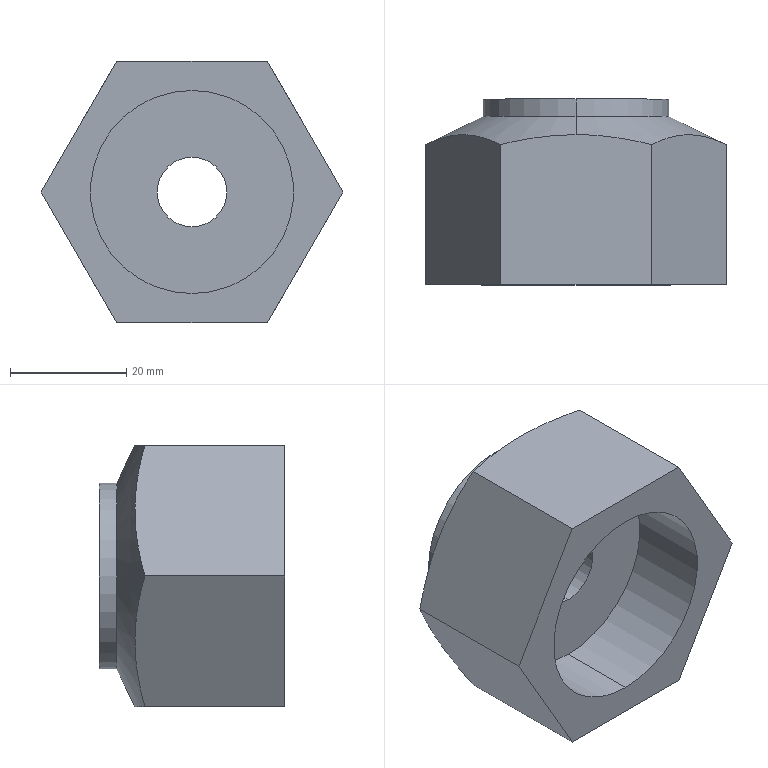Part | SolidWorks | features ICE 7 | 1 solid | 20 faces | box 51.962 x 32 x 45 mm | volume 33727 mm3 | plane 10 | cylinder 8 | cone 2 | commonest cylinder face diameters 12 x2 18 x2 32 x2 35 x2
STEP:
#1=CARTESIAN_POINT('',(0.,5.,-16.));
#2=VERTEX_POINT('',#1);
#3=CARTESIAN_POINT('',(0.,5.,16.));
#4=VERTEX_POINT('',#3);
#5=CARTESIAN_POINT('',(0.,5.,0.));
#6=DIRECTION('',(0.,1.,0.));
#7=DIRECTION('',(0.,0.,1.));
#8=AXIS2_PLACEMENT_3D('',#5,#6,#7);
#9=CIRCLE('',#8,16.);
#10=EDGE_CURVE('',#2,#4,#9,.T.);
#11=ORIENTED_EDGE('',*,*,#10,.F.);
#12=CARTESIAN_POINT('',(0.,1.83,-22.5));
#13=VERTEX_POINT('',#12);
#14=CARTESIAN_POINT('',(0.,5.,-16.));
#15=DIRECTION('',(0.,-0.4384,-0.8988));
#16=VECTOR('',#15,1000.);
#17=LINE('',#14,#16);
#18=EDGE_CURVE('',#2,#13,#17,.T.);
#19=ORIENTED_EDGE('',*,*,#18,.T.);
#20=CARTESIAN_POINT('',(-12.99,0.1321,-22.5));
#21=VERTEX_POINT('',#20);
#22=CARTESIAN_POINT('',(0.,1.83,-22.5));
#23=CARTESIAN_POINT('',(-2.167,1.83,-22.5));
#24=CARTESIAN_POINT('',(-4.338,1.674,-22.5));
#25=CARTESIAN_POINT('',(-7.601,1.232,-22.5));
#26=CARTESIAN_POINT('',(-8.692,1.049,-22.5));
#27=CARTESIAN_POINT('',(-10.854,0.6291,-22.5));
#28=CARTESIAN_POINT('',(-11.926,0.3916,-22.5));
#29=CARTESIAN_POINT('',(-12.99,0.1321,-22.5));
#30=B_SPLINE_CURVE_WITH_KNOTS('',3,(#22,#23,#24,#25,#26,#27,#28,#29),.UNSPECIFIED.,.F.,.F.,(4,2,2,4),(0.04128,0.04785,0.05113,0.05441),.UNSPECIFIED.);
#31=EDGE_CURVE('',#13,#21,#30,.T.);
#32=ORIENTED_EDGE('',*,*,#31,.T.);
#33=CARTESIAN_POINT('',(-25.981,0.1321,0.));
#34=VERTEX_POINT('',#33);
#35=CARTESIAN_POINT('',(-12.99,0.1321,-22.5));
#36=CARTESIAN_POINT('',(-14.059,0.6531,-20.65));
#37=CARTESIAN_POINT('',(-15.13,1.079,-18.793));
#38=CARTESIAN_POINT('',(-17.284,1.667,-15.062));
#39=CARTESIAN_POINT('',(-18.367,1.827,-13.188));
#40=CARTESIAN_POINT('',(-19.999,1.831,-10.361));
#41=CARTESIAN_POINT('',(-20.545,1.794,-9.416));
#42=CARTESIAN_POINT('',(-21.639,1.643,-7.521));
#43=CARTESIAN_POINT('',(-22.189,1.529,-6.568));
#44=CARTESIAN_POINT('',(-23.828,1.085,-3.729));
#45=CARTESIAN_POINT('',(-24.909,0.655,-1.857));
#46=CARTESIAN_POINT('',(-25.981,0.1321,0.));
#47=B_SPLINE_CURVE_WITH_KNOTS('',3,(#35,#36,#37,#38,#39,#40,#41,#42,#43,#44,#45,#46),.UNSPECIFIED.,.F.,.F.,(4,2,2,2,2,4),(0.000000235,0.006511,0.01302,0.01628,0.01953,0.02604),.UNSPECIFIED.);
#48=EDGE_CURVE('',#21,#34,#47,.T.);
#49=ORIENTED_EDGE('',*,*,#48,.T.);
#50=CARTESIAN_POINT('',(-12.99,0.1321,22.5));
#51=VERTEX_POINT('',#50);
#52=CARTESIAN_POINT('',(-25.981,0.1321,0.));
#53=CARTESIAN_POINT('',(-24.913,0.6531,1.85));
#54=CARTESIAN_POINT('',(-23.841,1.079,3.707));
#55=CARTESIAN_POINT('',(-21.687,1.667,7.438));
#56=CARTESIAN_POINT('',(-20.605,1.827,9.312));
#57=CARTESIAN_POINT('',(-18.972,1.831,12.139));
#58=CARTESIAN_POINT('',(-18.427,1.794,13.084));
#59=CARTESIAN_POINT('',(-17.332,1.643,14.979));
#60=CARTESIAN_POINT('',(-16.782,1.529,15.932));
#61=CARTESIAN_POINT('',(-15.143,1.085,18.771));
#62=CARTESIAN_POINT('',(-14.063,0.655,20.643));
#63=CARTESIAN_POINT('',(-12.99,0.1321,22.5));
#64=B_SPLINE_CURVE_WITH_KNOTS('',3,(#52,#53,#54,#55,#56,#57,#58,#59,#60,#61,#62,#63),.UNSPECIFIED.,.F.,.F.,(4,2,2,2,2,4),(0.000000235,0.006511,0.01302,0.01628,0.01953,0.02604),.UNSPECIFIED.);
#65=EDGE_CURVE('',#34,#51,#64,.T.);
#66=ORIENTED_EDGE('',*,*,#65,.T.);
#67=CARTESIAN_POINT('',(0.,1.83,22.5));
#68=VERTEX_POINT('',#67);
#69=CARTESIAN_POINT('',(-12.99,0.1321,22.5));
#70=CARTESIAN_POINT('',(-11.918,0.3935,22.5));
#71=CARTESIAN_POINT('',(-10.836,0.633,22.5));
#72=CARTESIAN_POINT('',(-8.674,1.052,22.5));
#73=CARTESIAN_POINT('',(-7.592,1.233,22.5));
#74=CARTESIAN_POINT('',(-4.344,1.673,22.5));
#75=CARTESIAN_POINT('',(-2.174,1.83,22.5));
#76=CARTESIAN_POINT('',(0.,1.83,22.5));
#77=B_SPLINE_CURVE_WITH_KNOTS('',3,(#69,#70,#71,#72,#73,#74,#75,#76),.UNSPECIFIED.,.F.,.F.,(4,2,2,4),(0.0281,0.0314,0.03469,0.04128),.UNSPECIFIED.);
#78=EDGE_CURVE('',#51,#68,#77,.T.);
#79=ORIENTED_EDGE('',*,*,#78,.T.);
#80=CARTESIAN_POINT('',(0.,5.,16.));
#81=DIRECTION('',(0.,-0.4384,0.8988));
#82=VECTOR('',#81,1000.);
#83=LINE('',#80,#82);
#84=EDGE_CURVE('',#4,#68,#83,.T.);
#85=ORIENTED_EDGE('',*,*,#84,.F.);
#86=EDGE_LOOP('',(#11,#19,#32,#49,#66,#79,#85));
#87=FACE_OUTER_BOUND('',#86,.T.);
#88=CARTESIAN_POINT('',(0.,5.,0.));
#89=DIRECTION('',(0.,-1.,0.));
#90=DIRECTION('',(0.,0.,1.));
#91=AXIS2_PLACEMENT_3D('',#88,#89,#90);
#92=CONICAL_SURFACE('',#91,16.,1.117);
#93=ADVANCED_FACE('',(#87),#92,.T.);
#94=CARTESIAN_POINT('',(0.,-7.,-9.));
#95=VERTEX_POINT('',#94);
#96=CARTESIAN_POINT('',(0.,-7.,9.));
#97=VERTEX_POINT('',#96);
#98=CARTESIAN_POINT('',(0.,-7.,0.));
#99=DIRECTION('',(0.,1.,0.));
#100=DIRECTION('',(0.,0.,1.));
#101=AXIS2_PLACEMENT_3D('',#98,#99,#100);
#102=CIRCLE('',#101,9.);
#103=EDGE_CURVE('',#95,#97,#102,.T.);
#104=ORIENTED_EDGE('',*,*,#103,.F.);
#105=CARTESIAN_POINT('',(0.,8.,-9.));
#106=VERTEX_POINT('',#105);
#107=CARTESIAN_POINT('',(0.,-7.,-9.));
#108=DIRECTION('',(0.,1.,0.));
#109=VECTOR('',#108,1000.);
#110=LINE('',#107,#109);
#111=EDGE_CURVE('',#95,#106,#110,.T.);
#112=ORIENTED_EDGE('',*,*,#111,.T.);
#113=CARTESIAN_POINT('',(0.,8.,9.));
#114=VERTEX_POINT('',#113);
#115=CARTESIAN_POINT('',(0.,8.,0.));
#116=DIRECTION('',(0.,1.,0.));
#117=DIRECTION('',(0.,0.,1.));
#118=AXIS2_PLACEMENT_3D('',#115,#116,#117);
#119=CIRCLE('',#118,9.);
#120=EDGE_CURVE('',#106,#114,#119,.T.);
#121=ORIENTED_EDGE('',*,*,#120,.T.);
#122=CARTESIAN_POINT('',(0.,-7.,9.));
#123=DIRECTION('',(0.,1.,0.));
#124=VECTOR('',#123,1000.);
#125=LINE('',#122,#124);
#126=EDGE_CURVE('',#97,#114,#125,.T.);
#127=ORIENTED_EDGE('',*,*,#126,.F.);
#128=EDGE_LOOP('',(#104,#112,#121,#127));
#129=FACE_OUTER_BOUND('',#128,.T.);
#130=CARTESIAN_POINT('',(0.,-7.,0.));
#131=DIRECTION('',(0.,1.,0.));
#132=DIRECTION('',(0.,0.,1.));
#133=AXIS2_PLACEMENT_3D('',#130,#131,#132);
#134=CYLINDRICAL_SURFACE('',#133,9.);
#135=ADVANCED_FACE('',(#129),#134,.F.);
#136=CARTESIAN_POINT('',(0.,8.,16.));
#137=VERTEX_POINT('',#136);
#138=CARTESIAN_POINT('',(0.,8.,-16.));
#139=VERTEX_POINT('',#138);
#140=CARTESIAN_POINT('',(0.,8.,0.));
#141=DIRECTION('',(0.,1.,0.));
#142=DIRECTION('',(0.,0.,1.));
#143=AXIS2_PLACEMENT_3D('',#140,#141,#142);
#144=CIRCLE('',#143,16.);
#145=EDGE_CURVE('',#137,#139,#144,.T.);
#146=ORIENTED_EDGE('',*,*,#145,.F.);
#147=CARTESIAN_POINT('',(0.,8.,16.));
#148=DIRECTION('',(0.,-1.,0.));
#149=VECTOR('',#148,1000.);
#150=LINE('',#147,#149);
#151=EDGE_CURVE('',#137,#4,#150,.T.);
#152=ORIENTED_EDGE('',*,*,#151,.T.);
#153=CARTESIAN_POINT('',(0.,5.,0.));
#154=DIRECTION('',(0.,1.,0.));
#155=DIRECTION('',(0.,0.,1.));
#156=AXIS2_PLACEMENT_3D('',#153,#154,#155);
#157=CIRCLE('',#156,16.);
#158=EDGE_CURVE('',#4,#2,#157,.T.);
#159=ORIENTED_EDGE('',*,*,#158,.T.);
#160=CARTESIAN_POINT('',(0.,8.,-16.));
#161=DIRECTION('',(0.,-1.,0.));
#162=VECTOR('',#161,1000.);
#163=LINE('',#160,#162);
#164=EDGE_CURVE('',#139,#2,#163,.T.);
#165=ORIENTED_EDGE('',*,*,#164,.F.);
#166=EDGE_LOOP('',(#146,#152,#159,#165));
#167=FACE_OUTER_BOUND('',#166,.T.);
#168=CARTESIAN_POINT('',(0.,8.,0.));
#169=DIRECTION('',(0.,-1.,0.));
#170=DIRECTION('',(0.,0.,-1.));
#171=AXIS2_PLACEMENT_3D('',#168,#169,#170);
#172=CYLINDRICAL_SURFACE('',#171,16.);
#173=ADVANCED_FACE('',(#167),#172,.T.);
#174=CARTESIAN_POINT('',(0.,-10.,17.5));
#175=VERTEX_POINT('',#174);
#176=CARTESIAN_POINT('',(0.,-10.,-17.5));
#177=VERTEX_POINT('',#176);
#178=CARTESIAN_POINT('',(0.,-10.,0.));
#179=DIRECTION('',(0.,-1.,0.));
#180=DIRECTION('',(0.,0.,-1.));
#181=AXIS2_PLACEMENT_3D('',#178,#179,#180);
#182=CIRCLE('',#181,17.5);
#183=EDGE_CURVE('',#175,#177,#182,.T.);
#184=ORIENTED_EDGE('',*,*,#183,.F.);
#185=CARTESIAN_POINT('',(0.,-24.,17.5));
#186=VERTEX_POINT('',#185);
#187=CARTESIAN_POINT('',(0.,-10.,17.5));
#188=DIRECTION('',(0.,-1.,0.));
#189=VECTOR('',#188,1000.);
#190=LINE('',#187,#189);
#191=EDGE_CURVE('',#175,#186,#190,.T.);
#192=ORIENTED_EDGE('',*,*,#191,.T.);
#193=CARTESIAN_POINT('',(0.,-24.,-17.5));
#194=VERTEX_POINT('',#193);
#195=CARTESIAN_POINT('',(0.,-24.,0.));
#196=DIRECTION('',(0.,-1.,0.));
#197=DIRECTION('',(0.,0.,-1.));
#198=AXIS2_PLACEMENT_3D('',#195,#196,#197);
#199=CIRCLE('',#198,17.5);
#200=EDGE_CURVE('',#186,#194,#199,.T.);
#201=ORIENTED_EDGE('',*,*,#200,.T.);
#202=CARTESIAN_POINT('',(0.,-10.,-17.5));
#203=DIRECTION('',(0.,-1.,0.));
#204=VECTOR('',#203,1000.);
#205=LINE('',#202,#204);
#206=EDGE_CURVE('',#177,#194,#205,.T.);
#207=ORIENTED_EDGE('',*,*,#206,.F.);
#208=EDGE_LOOP('',(#184,#192,#201,#207));
#209=FACE_OUTER_BOUND('',#208,.T.);
#210=CARTESIAN_POINT('',(0.,-10.,0.));
#211=DIRECTION('',(0.,-1.,0.));
#212=DIRECTION('',(0.,0.,-1.));
#213=AXIS2_PLACEMENT_3D('',#210,#211,#212);
#214=CYLINDRICAL_SURFACE('',#213,17.5);
#215=ADVANCED_FACE('',(#209),#214,.F.);
#216=CARTESIAN_POINT('',(0.,-7.,6.));
#217=VERTEX_POINT('',#216);
#218=CARTESIAN_POINT('',(0.,-7.,-6.));
#219=VERTEX_POINT('',#218);
#220=CARTESIAN_POINT('',(0.,-7.,0.));
#221=DIRECTION('',(0.,-1.,0.));
#222=DIRECTION('',(0.,0.,1.));
#223=AXIS2_PLACEMENT_3D('',#220,#221,#222);
#224=CIRCLE('',#223,6.);
#225=EDGE_CURVE('',#217,#219,#224,.T.);
#226=ORIENTED_EDGE('',*,*,#225,.F.);
#227=CARTESIAN_POINT('',(0.,-10.,6.));
#228=VERTEX_POINT('',#227);
#229=CARTESIAN_POINT('',(0.,8.,6.));
#230=DIRECTION('',(0.,-1.,0.));
#231=VECTOR('',#230,1000.);
#232=LINE('',#229,#231);
#233=EDGE_CURVE('',#217,#228,#232,.T.);
#234=ORIENTED_EDGE('',*,*,#233,.T.);
#235=CARTESIAN_POINT('',(0.,-10.,-6.));
#236=VERTEX_POINT('',#235);
#237=CARTESIAN_POINT('',(0.,-10.,0.));
#238=DIRECTION('',(0.,-1.,0.));
#239=DIRECTION('',(0.,0.,-1.));
#240=AXIS2_PLACEMENT_3D('',#237,#238,#239);
#241=CIRCLE('',#240,6.);
#242=EDGE_CURVE('',#228,#236,#241,.T.);
#243=ORIENTED_EDGE('',*,*,#242,.T.);
#244=CARTESIAN_POINT('',(0.,8.,-6.));
#245=DIRECTION('',(0.,-1.,0.));
#246=VECTOR('',#245,1000.);
#247=LINE('',#244,#246);
#248=EDGE_CURVE('',#219,#236,#247,.T.);
#249=ORIENTED_EDGE('',*,*,#248,.F.);
#250=EDGE_LOOP('',(#226,#234,#243,#249));
#251=FACE_OUTER_BOUND('',#250,.T.);
#252=CARTESIAN_POINT('',(0.,8.,0.));
#253=DIRECTION('',(0.,-1.,0.));
#254=DIRECTION('',(0.,0.,-1.));
#255=AXIS2_PLACEMENT_3D('',#252,#253,#254);
#256=CYLINDRICAL_SURFACE('',#255,6.);
#257=ADVANCED_FACE('',(#251),#256,.F.);
#258=ORIENTED_EDGE('',*,*,#65,.F.);
#259=CARTESIAN_POINT('',(-25.981,-24.,0.));
#260=VERTEX_POINT('',#259);
#261=CARTESIAN_POINT('',(-25.981,-24.,0.));
#262=DIRECTION('',(0.,1.,0.));
#263=VECTOR('',#262,1000.);
#264=LINE('',#261,#263);
#265=EDGE_CURVE('',#260,#34,#264,.T.);
#266=ORIENTED_EDGE('',*,*,#265,.F.);
#267=CARTESIAN_POINT('',(-12.99,-24.,22.5));
#268=VERTEX_POINT('',#267);
#269=CARTESIAN_POINT('',(-25.981,-24.,0.));
#270=DIRECTION('',(-0.5,0.,-0.866));
#271=VECTOR('',#270,1000.);
#272=LINE('',#269,#271);
#273=EDGE_CURVE('',#268,#260,#272,.T.);
#274=ORIENTED_EDGE('',*,*,#273,.F.);
#275=CARTESIAN_POINT('',(-12.99,-24.,22.5));
#276=DIRECTION('',(0.,1.,0.));
#277=VECTOR('',#276,1000.);
#278=LINE('',#275,#277);
#279=EDGE_CURVE('',#268,#51,#278,.T.);
#280=ORIENTED_EDGE('',*,*,#279,.T.);
#281=EDGE_LOOP('',(#258,#266,#274,#280));
#282=FACE_OUTER_BOUND('',#281,.T.);
#283=CARTESIAN_POINT('',(-25.981,-24.,0.));
#284=DIRECTION('',(0.866,0.,-0.5));
#285=DIRECTION('',(-0.5,0.,-0.866));
#286=AXIS2_PLACEMENT_3D('',#283,#284,#285);
#287=PLANE('',#286);
#288=ADVANCED_FACE('',(#282),#287,.F.);
#289=ORIENTED_EDGE('',*,*,#48,.F.);
#290=CARTESIAN_POINT('',(-12.99,-24.,-22.5));
#291=VERTEX_POINT('',#290);
#292=CARTESIAN_POINT('',(-12.99,-24.,-22.5));
#293=DIRECTION('',(0.,1.,0.));
#294=VECTOR('',#293,1000.);
#295=LINE('',#292,#294);
#296=EDGE_CURVE('',#291,#21,#295,.T.);
#297=ORIENTED_EDGE('',*,*,#296,.F.);
#298=CARTESIAN_POINT('',(-12.99,-24.,-22.5));
#299=DIRECTION('',(0.5,0.,-0.866));
#300=VECTOR('',#299,1000.);
#301=LINE('',#298,#300);
#302=EDGE_CURVE('',#260,#291,#301,.T.);
#303=ORIENTED_EDGE('',*,*,#302,.F.);
#304=ORIENTED_EDGE('',*,*,#265,.T.);
#305=EDGE_LOOP('',(#289,#297,#303,#304));
#306=FACE_OUTER_BOUND('',#305,.T.);
#307=CARTESIAN_POINT('',(-12.99,-24.,-22.5));
#308=DIRECTION('',(0.866,0.,0.5));
#309=DIRECTION('',(0.5,0.,-0.866));
#310=AXIS2_PLACEMENT_3D('',#307,#308,#309);
#311=PLANE('',#310);
#312=ADVANCED_FACE('',(#306),#311,.F.);
#313=CARTESIAN_POINT('',(12.99,0.1321,-22.5));
#314=VERTEX_POINT('',#313);
#315=CARTESIAN_POINT('',(12.99,0.1321,-22.5));
#316=CARTESIAN_POINT('',(11.918,0.3935,-22.5));
#317=CARTESIAN_POINT('',(10.836,0.633,-22.5));
#318=CARTESIAN_POINT('',(8.674,1.052,-22.5));
#319=CARTESIAN_POINT('',(7.592,1.233,-22.5));
#320=CARTESIAN_POINT('',(4.344,1.673,-22.5));
#321=CARTESIAN_POINT('',(2.174,1.83,-22.5));
#322=CARTESIAN_POINT('',(0.,1.83,-22.5));
#323=B_SPLINE_CURVE_WITH_KNOTS('',3,(#315,#316,#317,#318,#319,#320,#321,#322),.UNSPECIFIED.,.F.,.F.,(4,2,2,4),(0.0281,0.0314,0.03469,0.04128),.UNSPECIFIED.);
#324=EDGE_CURVE('',#314,#13,#323,.T.);
#325=ORIENTED_EDGE('',*,*,#324,.F.);
#326=CARTESIAN_POINT('',(12.99,-24.,-22.5));
#327=VERTEX_POINT('',#326);
#328=CARTESIAN_POINT('',(12.99,-24.,-22.5));
#329=DIRECTION('',(0.,1.,0.));
#330=VECTOR('',#329,1000.);
#331=LINE('',#328,#330);
#332=EDGE_CURVE('',#327,#314,#331,.T.);
#333=ORIENTED_EDGE('',*,*,#332,.F.);
#334=CARTESIAN_POINT('',(12.99,-24.,-22.5));
#335=DIRECTION('',(1.,0.,0.));
#336=VECTOR('',#335,1000.);
#337=LINE('',#334,#336);
#338=EDGE_CURVE('',#291,#327,#337,.T.);
#339=ORIENTED_EDGE('',*,*,#338,.F.);
#340=ORIENTED_EDGE('',*,*,#296,.T.);
#341=ORIENTED_EDGE('',*,*,#31,.F.);
#342=EDGE_LOOP('',(#325,#333,#339,#340,#341));
#343=FACE_OUTER_BOUND('',#342,.T.);
#344=CARTESIAN_POINT('',(12.99,-24.,-22.5));
#345=DIRECTION('',(0.,0.,1.));
#346=DIRECTION('',(1.,0.,0.));
#347=AXIS2_PLACEMENT_3D('',#344,#345,#346);
#348=PLANE('',#347);
#349=ADVANCED_FACE('',(#343),#348,.F.);
#350=CARTESIAN_POINT('',(25.981,0.1321,0.));
#351=VERTEX_POINT('',#350);
#352=CARTESIAN_POINT('',(25.981,0.1321,0.));
#353=CARTESIAN_POINT('',(24.913,0.6531,-1.85));
#354=CARTESIAN_POINT('',(23.841,1.079,-3.707));
#355=CARTESIAN_POINT('',(21.687,1.667,-7.438));
#356=CARTESIAN_POINT('',(20.605,1.827,-9.312));
#357=CARTESIAN_POINT('',(18.972,1.831,-12.139));
#358=CARTESIAN_POINT('',(18.427,1.794,-13.084));
#359=CARTESIAN_POINT('',(17.332,1.643,-14.979));
#360=CARTESIAN_POINT('',(16.782,1.529,-15.932));
#361=CARTESIAN_POINT('',(15.143,1.085,-18.771));
#362=CARTESIAN_POINT('',(14.063,0.655,-20.643));
#363=CARTESIAN_POINT('',(12.99,0.1321,-22.5));
#364=B_SPLINE_CURVE_WITH_KNOTS('',3,(#352,#353,#354,#355,#356,#357,#358,#359,#360,#361,#362,#363),.UNSPECIFIED.,.F.,.F.,(4,2,2,2,2,4),(0.000000235,0.006511,0.01302,0.01628,0.01953,0.02604),.UNSPECIFIED.);
#365=EDGE_CURVE('',#351,#314,#364,.T.);
#366=ORIENTED_EDGE('',*,*,#365,.F.);
#367=CARTESIAN_POINT('',(25.981,-24.,0.));
#368=VERTEX_POINT('',#367);
#369=CARTESIAN_POINT('',(25.981,-24.,0.));
#370=DIRECTION('',(0.,1.,0.));
#371=VECTOR('',#370,1000.);
#372=LINE('',#369,#371);
#373=EDGE_CURVE('',#368,#351,#372,.T.);
#374=ORIENTED_EDGE('',*,*,#373,.F.);
#375=CARTESIAN_POINT('',(25.981,-24.,0.));
#376=DIRECTION('',(0.5,0.,0.866));
#377=VECTOR('',#376,1000.);
#378=LINE('',#375,#377);
#379=EDGE_CURVE('',#327,#368,#378,.T.);
#380=ORIENTED_EDGE('',*,*,#379,.F.);
#381=ORIENTED_EDGE('',*,*,#332,.T.);
#382=EDGE_LOOP('',(#366,#374,#380,#381));
#383=FACE_OUTER_BOUND('',#382,.T.);
#384=CARTESIAN_POINT('',(25.981,-24.,0.));
#385=DIRECTION('',(-0.866,0.,0.5));
#386=DIRECTION('',(0.5,0.,0.866));
#387=AXIS2_PLACEMENT_3D('',#384,#385,#386);
#388=PLANE('',#387);
#389=ADVANCED_FACE('',(#383),#388,.F.);
#390=CARTESIAN_POINT('',(12.99,0.1321,22.5));
#391=VERTEX_POINT('',#390);
#392=CARTESIAN_POINT('',(12.99,0.1321,22.5));
#393=CARTESIAN_POINT('',(14.059,0.6531,20.65));
#394=CARTESIAN_POINT('',(15.13,1.079,18.793));
#395=CARTESIAN_POINT('',(17.284,1.667,15.062));
#396=CARTESIAN_POINT('',(18.367,1.827,13.188));
#397=CARTESIAN_POINT('',(19.999,1.831,10.361));
#398=CARTESIAN_POINT('',(20.545,1.794,9.416));
#399=CARTESIAN_POINT('',(21.639,1.643,7.521));
#400=CARTESIAN_POINT('',(22.189,1.529,6.568));
#401=CARTESIAN_POINT('',(23.828,1.085,3.729));
#402=CARTESIAN_POINT('',(24.909,0.655,1.857));
#403=CARTESIAN_POINT('',(25.981,0.1321,0.));
#404=B_SPLINE_CURVE_WITH_KNOTS('',3,(#392,#393,#394,#395,#396,#397,#398,#399,#400,#401,#402,#403),.UNSPECIFIED.,.F.,.F.,(4,2,2,2,2,4),(0.000000235,0.006511,0.01302,0.01628,0.01953,0.02604),.UNSPECIFIED.);
#405=EDGE_CURVE('',#391,#351,#404,.T.);
#406=ORIENTED_EDGE('',*,*,#405,.F.);
#407=CARTESIAN_POINT('',(12.99,-24.,22.5));
#408=VERTEX_POINT('',#407);
#409=CARTESIAN_POINT('',(12.99,-24.,22.5));
#410=DIRECTION('',(0.,1.,0.));
#411=VECTOR('',#410,1000.);
#412=LINE('',#409,#411);
#413=EDGE_CURVE('',#408,#391,#412,.T.);
#414=ORIENTED_EDGE('',*,*,#413,.F.);
#415=CARTESIAN_POINT('',(12.99,-24.,22.5));
#416=DIRECTION('',(-0.5,0.,0.866));
#417=VECTOR('',#416,1000.);
#418=LINE('',#415,#417);
#419=EDGE_CURVE('',#368,#408,#418,.T.);
#420=ORIENTED_EDGE('',*,*,#419,.F.);
#421=ORIENTED_EDGE('',*,*,#373,.T.);
#422=EDGE_LOOP('',(#406,#414,#420,#421));
#423=FACE_OUTER_BOUND('',#422,.T.);
#424=CARTESIAN_POINT('',(12.99,-24.,22.5));
#425=DIRECTION('',(-0.866,0.,-0.5));
#426=DIRECTION('',(-0.5,0.,0.866));
#427=AXIS2_PLACEMENT_3D('',#424,#425,#426);
#428=PLANE('',#427);
#429=ADVANCED_FACE('',(#423),#428,.F.);
#430=ORIENTED_EDGE('',*,*,#78,.F.);
#431=ORIENTED_EDGE('',*,*,#279,.F.);
#432=CARTESIAN_POINT('',(-12.99,-24.,22.5));
#433=DIRECTION('',(-1.,0.,0.));
#434=VECTOR('',#433,1000.);
#435=LINE('',#432,#434);
#436=EDGE_CURVE('',#408,#268,#435,.T.);
#437=ORIENTED_EDGE('',*,*,#436,.F.);
#438=ORIENTED_EDGE('',*,*,#413,.T.);
#439=CARTESIAN_POINT('',(0.,1.83,22.5));
#440=CARTESIAN_POINT('',(2.167,1.83,22.5));
#441=CARTESIAN_POINT('',(4.338,1.674,22.5));
#442=CARTESIAN_POINT('',(7.601,1.232,22.5));
#443=CARTESIAN_POINT('',(8.692,1.049,22.5));
#444=CARTESIAN_POINT('',(10.854,0.6291,22.5));
#445=CARTESIAN_POINT('',(11.926,0.3916,22.5));
#446=CARTESIAN_POINT('',(12.99,0.1321,22.5));
#447=B_SPLINE_CURVE_WITH_KNOTS('',3,(#439,#440,#441,#442,#443,#444,#445,#446),.UNSPECIFIED.,.F.,.F.,(4,2,2,4),(0.04128,0.04785,0.05113,0.05441),.UNSPECIFIED.);
#448=EDGE_CURVE('',#68,#391,#447,.T.);
#449=ORIENTED_EDGE('',*,*,#448,.F.);
#450=EDGE_LOOP('',(#430,#431,#437,#438,#449));
#451=FACE_OUTER_BOUND('',#450,.T.);
#452=CARTESIAN_POINT('',(-12.99,-24.,22.5));
#453=DIRECTION('',(0.,0.,-1.));
#454=DIRECTION('',(-1.,0.,0.));
#455=AXIS2_PLACEMENT_3D('',#452,#453,#454);
#456=PLANE('',#455);
#457=ADVANCED_FACE('',(#451),#456,.F.);
#458=ORIENTED_EDGE('',*,*,#233,.F.);
#459=CARTESIAN_POINT('',(0.,-7.,0.));
#460=DIRECTION('',(0.,-1.,0.));
#461=DIRECTION('',(0.,0.,1.));
#462=AXIS2_PLACEMENT_3D('',#459,#460,#461);
#463=CIRCLE('',#462,6.);
#464=EDGE_CURVE('',#219,#217,#463,.T.);
#465=ORIENTED_EDGE('',*,*,#464,.F.);
#466=ORIENTED_EDGE('',*,*,#248,.T.);
#467=CARTESIAN_POINT('',(0.,-10.,0.));
#468=DIRECTION('',(0.,-1.,0.));
#469=DIRECTION('',(0.,0.,-1.));
#470=AXIS2_PLACEMENT_3D('',#467,#468,#469);
#471=CIRCLE('',#470,6.);
#472=EDGE_CURVE('',#236,#228,#471,.T.);
#473=ORIENTED_EDGE('',*,*,#472,.T.);
#474=EDGE_LOOP('',(#458,#465,#466,#473));
#475=FACE_OUTER_BOUND('',#474,.T.);
#476=CARTESIAN_POINT('',(0.,8.,0.));
#477=DIRECTION('',(0.,-1.,0.));
#478=DIRECTION('',(0.,0.,-1.));
#479=AXIS2_PLACEMENT_3D('',#476,#477,#478);
#480=CYLINDRICAL_SURFACE('',#479,6.);
#481=ADVANCED_FACE('',(#475),#480,.F.);
#482=CARTESIAN_POINT('',(0.,-24.,0.));
#483=DIRECTION('',(0.,-1.,0.));
#484=DIRECTION('',(0.,0.,-1.));
#485=AXIS2_PLACEMENT_3D('',#482,#483,#484);
#486=CIRCLE('',#485,17.5);
#487=EDGE_CURVE('',#194,#186,#486,.T.);
#488=ORIENTED_EDGE('',*,*,#487,.F.);
#489=ORIENTED_EDGE('',*,*,#200,.F.);
#490=EDGE_LOOP('',(#488,#489));
#491=FACE_BOUND('',#490,.T.);
#492=ORIENTED_EDGE('',*,*,#273,.T.);
#493=ORIENTED_EDGE('',*,*,#302,.T.);
#494=ORIENTED_EDGE('',*,*,#338,.T.);
#495=ORIENTED_EDGE('',*,*,#379,.T.);
#496=ORIENTED_EDGE('',*,*,#419,.T.);
#497=ORIENTED_EDGE('',*,*,#436,.T.);
#498=EDGE_LOOP('',(#492,#493,#494,#495,#496,#497));
#499=FACE_OUTER_BOUND('',#498,.T.);
#500=CARTESIAN_POINT('',(0.,-24.,0.));
#501=DIRECTION('',(0.,1.,0.));
#502=DIRECTION('',(0.,0.,1.));
#503=AXIS2_PLACEMENT_3D('',#500,#501,#502);
#504=PLANE('',#503);
#505=ADVANCED_FACE('',(#491,#499),#504,.F.);
#506=ORIENTED_EDGE('',*,*,#191,.F.);
#507=CARTESIAN_POINT('',(0.,-10.,0.));
#508=DIRECTION('',(0.,-1.,0.));
#509=DIRECTION('',(0.,0.,-1.));
#510=AXIS2_PLACEMENT_3D('',#507,#508,#509);
#511=CIRCLE('',#510,17.5);
#512=EDGE_CURVE('',#177,#175,#511,.T.);
#513=ORIENTED_EDGE('',*,*,#512,.F.);
#514=ORIENTED_EDGE('',*,*,#206,.T.);
#515=ORIENTED_EDGE('',*,*,#487,.T.);
#516=EDGE_LOOP('',(#506,#513,#514,#515));
#517=FACE_OUTER_BOUND('',#516,.T.);
#518=CARTESIAN_POINT('',(0.,-10.,0.));
#519=DIRECTION('',(0.,-1.,0.));
#520=DIRECTION('',(0.,0.,-1.));
#521=AXIS2_PLACEMENT_3D('',#518,#519,#520);
#522=CYLINDRICAL_SURFACE('',#521,17.5);
#523=ADVANCED_FACE('',(#517),#522,.F.);
#524=ORIENTED_EDGE('',*,*,#512,.T.);
#525=ORIENTED_EDGE('',*,*,#183,.T.);
#526=EDGE_LOOP('',(#524,#525));
#527=FACE_OUTER_BOUND('',#526,.T.);
#528=ORIENTED_EDGE('',*,*,#472,.F.);
#529=ORIENTED_EDGE('',*,*,#242,.F.);
#530=EDGE_LOOP('',(#528,#529));
#531=FACE_BOUND('',#530,.T.);
#532=CARTESIAN_POINT('',(0.,-10.,0.));
#533=DIRECTION('',(0.,-1.,0.));
#534=DIRECTION('',(0.,0.,-1.));
#535=AXIS2_PLACEMENT_3D('',#532,#533,#534);
#536=PLANE('',#535);
#537=ADVANCED_FACE('',(#527,#531),#536,.T.);
#538=CARTESIAN_POINT('',(0.,8.,0.));
#539=DIRECTION('',(0.,1.,0.));
#540=DIRECTION('',(0.,0.,1.));
#541=AXIS2_PLACEMENT_3D('',#538,#539,#540);
#542=CIRCLE('',#541,9.);
#543=EDGE_CURVE('',#114,#106,#542,.T.);
#544=ORIENTED_EDGE('',*,*,#543,.F.);
#545=ORIENTED_EDGE('',*,*,#120,.F.);
#546=EDGE_LOOP('',(#544,#545));
#547=FACE_BOUND('',#546,.T.);
#548=CARTESIAN_POINT('',(0.,8.,0.));
#549=DIRECTION('',(0.,1.,0.));
#550=DIRECTION('',(0.,0.,1.));
#551=AXIS2_PLACEMENT_3D('',#548,#549,#550);
#552=CIRCLE('',#551,16.);
#553=EDGE_CURVE('',#139,#137,#552,.T.);
#554=ORIENTED_EDGE('',*,*,#553,.T.);
#555=ORIENTED_EDGE('',*,*,#145,.T.);
#556=EDGE_LOOP('',(#554,#555));
#557=FACE_OUTER_BOUND('',#556,.T.);
#558=CARTESIAN_POINT('',(0.,8.,0.));
#559=DIRECTION('',(0.,1.,0.));
#560=DIRECTION('',(0.,0.,1.));
#561=AXIS2_PLACEMENT_3D('',#558,#559,#560);
#562=PLANE('',#561);
#563=ADVANCED_FACE('',(#547,#557),#562,.T.);
#564=ORIENTED_EDGE('',*,*,#151,.F.);
#565=ORIENTED_EDGE('',*,*,#553,.F.);
#566=ORIENTED_EDGE('',*,*,#164,.T.);
#567=ORIENTED_EDGE('',*,*,#10,.T.);
#568=EDGE_LOOP('',(#564,#565,#566,#567));
#569=FACE_OUTER_BOUND('',#568,.T.);
#570=CARTESIAN_POINT('',(0.,8.,0.));
#571=DIRECTION('',(0.,-1.,0.));
#572=DIRECTION('',(0.,0.,-1.));
#573=AXIS2_PLACEMENT_3D('',#570,#571,#572);
#574=CYLINDRICAL_SURFACE('',#573,16.);
#575=ADVANCED_FACE('',(#569),#574,.T.);
#576=CARTESIAN_POINT('',(0.,-7.,0.));
#577=DIRECTION('',(0.,1.,0.));
#578=DIRECTION('',(0.,0.,1.));
#579=AXIS2_PLACEMENT_3D('',#576,#577,#578);
#580=CIRCLE('',#579,9.);
#581=EDGE_CURVE('',#97,#95,#580,.T.);
#582=ORIENTED_EDGE('',*,*,#581,.T.);
#583=ORIENTED_EDGE('',*,*,#103,.T.);
#584=EDGE_LOOP('',(#582,#583));
#585=FACE_OUTER_BOUND('',#584,.T.);
#586=ORIENTED_EDGE('',*,*,#464,.T.);
#587=ORIENTED_EDGE('',*,*,#225,.T.);
#588=EDGE_LOOP('',(#586,#587));
#589=FACE_BOUND('',#588,.T.);
#590=CARTESIAN_POINT('',(0.,-7.,0.));
#591=DIRECTION('',(0.,1.,0.));
#592=DIRECTION('',(0.,0.,1.));
#593=AXIS2_PLACEMENT_3D('',#590,#591,#592);
#594=PLANE('',#593);
#595=ADVANCED_FACE('',(#585,#589),#594,.T.);
#596=ORIENTED_EDGE('',*,*,#111,.F.);
#597=ORIENTED_EDGE('',*,*,#581,.F.);
#598=ORIENTED_EDGE('',*,*,#126,.T.);
#599=ORIENTED_EDGE('',*,*,#543,.T.);
#600=EDGE_LOOP('',(#596,#597,#598,#599));
#601=FACE_OUTER_BOUND('',#600,.T.);
#602=CARTESIAN_POINT('',(0.,-7.,0.));
#603=DIRECTION('',(0.,1.,0.));
#604=DIRECTION('',(0.,0.,1.));
#605=AXIS2_PLACEMENT_3D('',#602,#603,#604);
#606=CYLINDRICAL_SURFACE('',#605,9.);
#607=ADVANCED_FACE('',(#601),#606,.F.);
#608=ORIENTED_EDGE('',*,*,#18,.F.);
#609=ORIENTED_EDGE('',*,*,#158,.F.);
#610=ORIENTED_EDGE('',*,*,#84,.T.);
#611=ORIENTED_EDGE('',*,*,#448,.T.);
#612=ORIENTED_EDGE('',*,*,#405,.T.);
#613=ORIENTED_EDGE('',*,*,#365,.T.);
#614=ORIENTED_EDGE('',*,*,#324,.T.);
#615=EDGE_LOOP('',(#608,#609,#610,#611,#612,#613,#614));
#616=FACE_OUTER_BOUND('',#615,.T.);
#617=CARTESIAN_POINT('',(0.,5.,0.));
#618=DIRECTION('',(0.,-1.,0.));
#619=DIRECTION('',(0.,0.,1.));
#620=AXIS2_PLACEMENT_3D('',#617,#618,#619);
#621=CONICAL_SURFACE('',#620,16.,1.117);
#622=ADVANCED_FACE('',(#616),#621,.T.);
#623=CLOSED_SHELL('',(#93,#135,#173,#215,#257,#288,#312,#349,#389,#429,#457,#481,#505,#523,#537,#563,#575,#595,#607,#622));
#624=MANIFOLD_SOLID_BREP('',#623);
#625=CARTESIAN_POINT('',(0.,0.,0.));
#626=DIRECTION('',(0.,0.,1.));
#627=DIRECTION('',(1.,0.,0.));
#628=AXIS2_PLACEMENT_3D('',#625,#626,#627);
#629=(LENGTH_UNIT()NAMED_UNIT(*)SI_UNIT(.MILLI.,.METRE.));
#630=UNCERTAINTY_MEASURE_WITH_UNIT(LENGTH_MEASURE(0.00001),#629,'','');
#631=(NAMED_UNIT(*)PLANE_ANGLE_UNIT()SI_UNIT($,.RADIAN.));
#632=(NAMED_UNIT(*)SI_UNIT($,.STERADIAN.)SOLID_ANGLE_UNIT());
#633=(GEOMETRIC_REPRESENTATION_CONTEXT(3)GLOBAL_UNCERTAINTY_ASSIGNED_CONTEXT((#630))GLOBAL_UNIT_ASSIGNED_CONTEXT((#629,#631,#632))REPRESENTATION_CONTEXT('',''));
#634=ADVANCED_BREP_SHAPE_REPRESENTATION('',(#624,#628),#633);